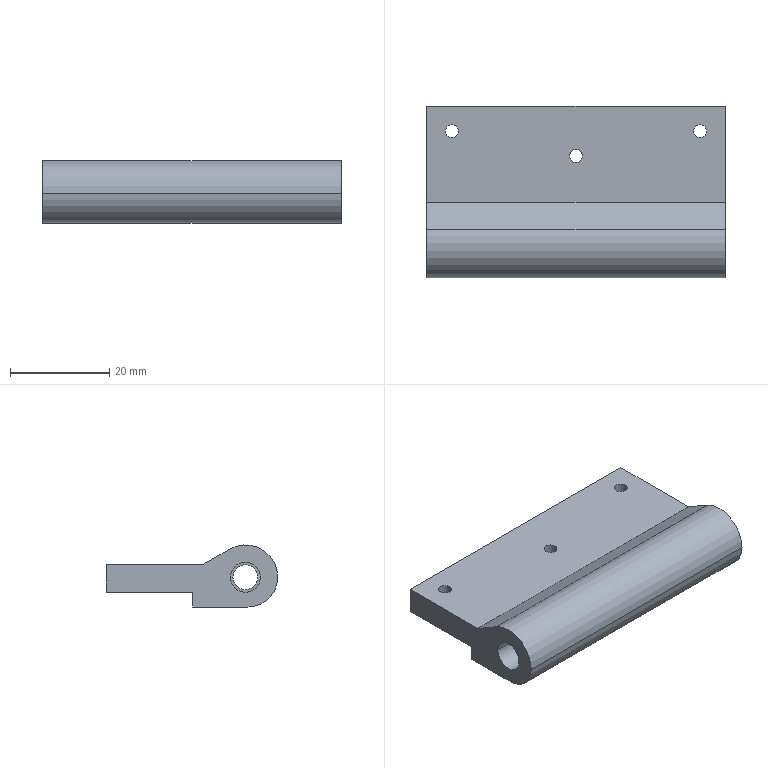Part | NX | 1 solid | 30 faces | box 60 x 34.5 x 12.5 mm | volume 14807 mm3 | cylinder 14 | plane 10 | cone 6 | commonest cylinder face diameters 2.6 x6 6.02 x4 5 x2 12 x1 13 x1
STEP:
#1=CARTESIAN_POINT('',(-23.7,12.25,-4.));
#2=VERTEX_POINT('',#1);
#3=CARTESIAN_POINT('',(-26.3,12.25,-4.));
#4=VERTEX_POINT('',#3);
#5=CARTESIAN_POINT('',(-25.,12.25,-4.));
#6=DIRECTION('',(0.,0.,1.));
#7=DIRECTION('',(1.,0.,0.));
#8=AXIS2_PLACEMENT_3D('',#5,#6,#7);
#9=CIRCLE('',#8,1.3);
#10=EDGE_CURVE('',#2,#4,#9,.T.);
#11=ORIENTED_EDGE('',*,*,#10,.T.);
#12=CARTESIAN_POINT('',(-26.3,12.25,-9.));
#13=VERTEX_POINT('',#12);
#14=CARTESIAN_POINT('',(-26.3,12.25,-10.5));
#15=DIRECTION('',(0.,0.,-1.));
#16=VECTOR('',#15,1000.);
#17=LINE('',#14,#16);
#18=EDGE_CURVE('',#4,#13,#17,.T.);
#19=ORIENTED_EDGE('',*,*,#18,.T.);
#20=CARTESIAN_POINT('',(-23.7,12.25,-9.));
#21=VERTEX_POINT('',#20);
#22=CARTESIAN_POINT('',(-25.,12.25,-9.));
#23=DIRECTION('',(0.,0.,1.));
#24=DIRECTION('',(1.,0.,0.));
#25=AXIS2_PLACEMENT_3D('',#22,#23,#24);
#26=CIRCLE('',#25,1.3);
#27=EDGE_CURVE('',#21,#13,#26,.T.);
#28=ORIENTED_EDGE('',*,*,#27,.F.);
#29=CARTESIAN_POINT('',(-23.7,12.25,-10.5));
#30=DIRECTION('',(0.,0.,-1.));
#31=VECTOR('',#30,1000.);
#32=LINE('',#29,#31);
#33=EDGE_CURVE('',#2,#21,#32,.T.);
#34=ORIENTED_EDGE('',*,*,#33,.F.);
#35=EDGE_LOOP('',(#11,#19,#28,#34));
#36=FACE_BOUND('',#35,.T.);
#37=CARTESIAN_POINT('',(-25.,12.25,-10.5));
#38=DIRECTION('',(0.,0.,-1.));
#39=DIRECTION('',(-1.,0.,0.));
#40=AXIS2_PLACEMENT_3D('',#37,#38,#39);
#41=CYLINDRICAL_SURFACE('',#40,1.3);
#42=ADVANCED_FACE('',(#36),#41,.F.);
#43=CARTESIAN_POINT('',(1.3,7.25,-4.));
#44=VERTEX_POINT('',#43);
#45=CARTESIAN_POINT('',(-1.3,7.25,-4.));
#46=VERTEX_POINT('',#45);
#47=CARTESIAN_POINT('',(0.,7.25,-4.));
#48=DIRECTION('',(0.,0.,1.));
#49=DIRECTION('',(1.,0.,0.));
#50=AXIS2_PLACEMENT_3D('',#47,#48,#49);
#51=CIRCLE('',#50,1.3);
#52=EDGE_CURVE('',#44,#46,#51,.T.);
#53=ORIENTED_EDGE('',*,*,#52,.T.);
#54=CARTESIAN_POINT('',(-1.3,7.25,-9.));
#55=VERTEX_POINT('',#54);
#56=CARTESIAN_POINT('',(-1.3,7.25,-10.5));
#57=DIRECTION('',(0.,0.,-1.));
#58=VECTOR('',#57,1000.);
#59=LINE('',#56,#58);
#60=EDGE_CURVE('',#46,#55,#59,.T.);
#61=ORIENTED_EDGE('',*,*,#60,.T.);
#62=CARTESIAN_POINT('',(1.3,7.25,-9.));
#63=VERTEX_POINT('',#62);
#64=CARTESIAN_POINT('',(0.,7.25,-9.));
#65=DIRECTION('',(0.,0.,1.));
#66=DIRECTION('',(1.,0.,0.));
#67=AXIS2_PLACEMENT_3D('',#64,#65,#66);
#68=CIRCLE('',#67,1.3);
#69=EDGE_CURVE('',#63,#55,#68,.T.);
#70=ORIENTED_EDGE('',*,*,#69,.F.);
#71=CARTESIAN_POINT('',(1.3,7.25,-10.5));
#72=DIRECTION('',(0.,0.,-1.));
#73=VECTOR('',#72,1000.);
#74=LINE('',#71,#73);
#75=EDGE_CURVE('',#44,#63,#74,.T.);
#76=ORIENTED_EDGE('',*,*,#75,.F.);
#77=EDGE_LOOP('',(#53,#61,#70,#76));
#78=FACE_BOUND('',#77,.T.);
#79=CARTESIAN_POINT('',(0.,7.25,-10.5));
#80=DIRECTION('',(0.,0.,-1.));
#81=DIRECTION('',(-1.,0.,0.));
#82=AXIS2_PLACEMENT_3D('',#79,#80,#81);
#83=CYLINDRICAL_SURFACE('',#82,1.3);
#84=ADVANCED_FACE('',(#78),#83,.F.);
#85=CARTESIAN_POINT('',(26.3,12.25,-4.));
#86=VERTEX_POINT('',#85);
#87=CARTESIAN_POINT('',(23.7,12.25,-4.));
#88=VERTEX_POINT('',#87);
#89=CARTESIAN_POINT('',(25.,12.25,-4.));
#90=DIRECTION('',(0.,0.,1.));
#91=DIRECTION('',(1.,0.,0.));
#92=AXIS2_PLACEMENT_3D('',#89,#90,#91);
#93=CIRCLE('',#92,1.3);
#94=EDGE_CURVE('',#86,#88,#93,.T.);
#95=ORIENTED_EDGE('',*,*,#94,.T.);
#96=CARTESIAN_POINT('',(23.7,12.25,-9.));
#97=VERTEX_POINT('',#96);
#98=CARTESIAN_POINT('',(23.7,12.25,-10.5));
#99=DIRECTION('',(0.,0.,-1.));
#100=VECTOR('',#99,1000.);
#101=LINE('',#98,#100);
#102=EDGE_CURVE('',#88,#97,#101,.T.);
#103=ORIENTED_EDGE('',*,*,#102,.T.);
#104=CARTESIAN_POINT('',(26.3,12.25,-9.));
#105=VERTEX_POINT('',#104);
#106=CARTESIAN_POINT('',(25.,12.25,-9.));
#107=DIRECTION('',(0.,0.,1.));
#108=DIRECTION('',(1.,0.,0.));
#109=AXIS2_PLACEMENT_3D('',#106,#107,#108);
#110=CIRCLE('',#109,1.3);
#111=EDGE_CURVE('',#105,#97,#110,.T.);
#112=ORIENTED_EDGE('',*,*,#111,.F.);
#113=CARTESIAN_POINT('',(26.3,12.25,-10.5));
#114=DIRECTION('',(0.,0.,-1.));
#115=VECTOR('',#114,1000.);
#116=LINE('',#113,#115);
#117=EDGE_CURVE('',#86,#105,#116,.T.);
#118=ORIENTED_EDGE('',*,*,#117,.F.);
#119=EDGE_LOOP('',(#95,#103,#112,#118));
#120=FACE_BOUND('',#119,.T.);
#121=CARTESIAN_POINT('',(25.,12.25,-10.5));
#122=DIRECTION('',(0.,0.,-1.));
#123=DIRECTION('',(-1.,0.,0.));
#124=AXIS2_PLACEMENT_3D('',#121,#122,#123);
#125=CYLINDRICAL_SURFACE('',#124,1.3);
#126=ADVANCED_FACE('',(#120),#125,.F.);
#127=ORIENTED_EDGE('',*,*,#27,.T.);
#128=CARTESIAN_POINT('',(-26.8,12.25,-9.5));
#129=VERTEX_POINT('',#128);
#130=CARTESIAN_POINT('',(-26.8,12.25,-9.5));
#131=DIRECTION('',(-0.7071,0.,-0.7071));
#132=VECTOR('',#131,1000.);
#133=LINE('',#130,#132);
#134=EDGE_CURVE('',#13,#129,#133,.T.);
#135=ORIENTED_EDGE('',*,*,#134,.T.);
#136=CARTESIAN_POINT('',(-23.2,12.25,-9.5));
#137=VERTEX_POINT('',#136);
#138=CARTESIAN_POINT('',(-25.,12.25,-9.5));
#139=DIRECTION('',(0.,0.,1.));
#140=DIRECTION('',(1.,0.,0.));
#141=AXIS2_PLACEMENT_3D('',#138,#139,#140);
#142=CIRCLE('',#141,1.8);
#143=EDGE_CURVE('',#137,#129,#142,.T.);
#144=ORIENTED_EDGE('',*,*,#143,.F.);
#145=CARTESIAN_POINT('',(-23.2,12.25,-9.5));
#146=DIRECTION('',(0.7071,0.,-0.7071));
#147=VECTOR('',#146,1000.);
#148=LINE('',#145,#147);
#149=EDGE_CURVE('',#21,#137,#148,.T.);
#150=ORIENTED_EDGE('',*,*,#149,.F.);
#151=EDGE_LOOP('',(#127,#135,#144,#150));
#152=FACE_BOUND('',#151,.T.);
#153=CARTESIAN_POINT('',(-25.,12.25,-9.5));
#154=DIRECTION('',(0.,0.,-1.));
#155=DIRECTION('',(-1.,0.,0.));
#156=AXIS2_PLACEMENT_3D('',#153,#154,#155);
#157=CONICAL_SURFACE('',#156,1.8,0.7854);
#158=ADVANCED_FACE('',(#152),#157,.F.);
#159=ORIENTED_EDGE('',*,*,#69,.T.);
#160=CARTESIAN_POINT('',(-1.8,7.25,-9.5));
#161=VERTEX_POINT('',#160);
#162=CARTESIAN_POINT('',(-1.8,7.25,-9.5));
#163=DIRECTION('',(-0.7071,0.,-0.7071));
#164=VECTOR('',#163,1000.);
#165=LINE('',#162,#164);
#166=EDGE_CURVE('',#55,#161,#165,.T.);
#167=ORIENTED_EDGE('',*,*,#166,.T.);
#168=CARTESIAN_POINT('',(1.8,7.25,-9.5));
#169=VERTEX_POINT('',#168);
#170=CARTESIAN_POINT('',(0.,7.25,-9.5));
#171=DIRECTION('',(0.,0.,1.));
#172=DIRECTION('',(1.,0.,0.));
#173=AXIS2_PLACEMENT_3D('',#170,#171,#172);
#174=CIRCLE('',#173,1.8);
#175=EDGE_CURVE('',#169,#161,#174,.T.);
#176=ORIENTED_EDGE('',*,*,#175,.F.);
#177=CARTESIAN_POINT('',(1.8,7.25,-9.5));
#178=DIRECTION('',(0.7071,0.,-0.7071));
#179=VECTOR('',#178,1000.);
#180=LINE('',#177,#179);
#181=EDGE_CURVE('',#63,#169,#180,.T.);
#182=ORIENTED_EDGE('',*,*,#181,.F.);
#183=EDGE_LOOP('',(#159,#167,#176,#182));
#184=FACE_BOUND('',#183,.T.);
#185=CARTESIAN_POINT('',(0.,7.25,-9.5));
#186=DIRECTION('',(0.,0.,-1.));
#187=DIRECTION('',(-1.,0.,0.));
#188=AXIS2_PLACEMENT_3D('',#185,#186,#187);
#189=CONICAL_SURFACE('',#188,1.8,0.7854);
#190=ADVANCED_FACE('',(#184),#189,.F.);
#191=ORIENTED_EDGE('',*,*,#111,.T.);
#192=CARTESIAN_POINT('',(23.2,12.25,-9.5));
#193=VERTEX_POINT('',#192);
#194=CARTESIAN_POINT('',(23.2,12.25,-9.5));
#195=DIRECTION('',(-0.7071,0.,-0.7071));
#196=VECTOR('',#195,1000.);
#197=LINE('',#194,#196);
#198=EDGE_CURVE('',#97,#193,#197,.T.);
#199=ORIENTED_EDGE('',*,*,#198,.T.);
#200=CARTESIAN_POINT('',(26.8,12.25,-9.5));
#201=VERTEX_POINT('',#200);
#202=CARTESIAN_POINT('',(25.,12.25,-9.5));
#203=DIRECTION('',(0.,0.,1.));
#204=DIRECTION('',(1.,0.,0.));
#205=AXIS2_PLACEMENT_3D('',#202,#203,#204);
#206=CIRCLE('',#205,1.8);
#207=EDGE_CURVE('',#201,#193,#206,.T.);
#208=ORIENTED_EDGE('',*,*,#207,.F.);
#209=CARTESIAN_POINT('',(26.8,12.25,-9.5));
#210=DIRECTION('',(0.7071,0.,-0.7071));
#211=VECTOR('',#210,1000.);
#212=LINE('',#209,#211);
#213=EDGE_CURVE('',#105,#201,#212,.T.);
#214=ORIENTED_EDGE('',*,*,#213,.F.);
#215=EDGE_LOOP('',(#191,#199,#208,#214));
#216=FACE_BOUND('',#215,.T.);
#217=CARTESIAN_POINT('',(25.,12.25,-9.5));
#218=DIRECTION('',(0.,0.,-1.));
#219=DIRECTION('',(-1.,0.,0.));
#220=AXIS2_PLACEMENT_3D('',#217,#218,#219);
#221=CONICAL_SURFACE('',#220,1.8,0.7854);
#222=ADVANCED_FACE('',(#216),#221,.F.);
#223=CARTESIAN_POINT('',(-30.,-13.76,-6.5));
#224=VERTEX_POINT('',#223);
#225=CARTESIAN_POINT('',(-30.,-7.74,-6.5));
#226=VERTEX_POINT('',#225);
#227=CARTESIAN_POINT('',(-30.,-10.75,-6.5));
#228=DIRECTION('',(-1.,0.,0.));
#229=DIRECTION('',(0.,-1.,0.));
#230=AXIS2_PLACEMENT_3D('',#227,#228,#229);
#231=CIRCLE('',#230,3.01);
#232=EDGE_CURVE('',#224,#226,#231,.T.);
#233=ORIENTED_EDGE('',*,*,#232,.T.);
#234=CARTESIAN_POINT('',(-20.2,-7.74,-6.5));
#235=VERTEX_POINT('',#234);
#236=CARTESIAN_POINT('',(-30.,-7.74,-6.5));
#237=DIRECTION('',(1.,0.,0.));
#238=VECTOR('',#237,1000.);
#239=LINE('',#236,#238);
#240=EDGE_CURVE('',#235,#226,#239,.F.);
#241=ORIENTED_EDGE('',*,*,#240,.F.);
#242=CARTESIAN_POINT('',(-20.2,-13.76,-6.5));
#243=VERTEX_POINT('',#242);
#244=CARTESIAN_POINT('',(-20.2,-10.75,-6.5));
#245=DIRECTION('',(-1.,0.,0.));
#246=DIRECTION('',(0.,-1.,0.));
#247=AXIS2_PLACEMENT_3D('',#244,#245,#246);
#248=CIRCLE('',#247,3.01);
#249=EDGE_CURVE('',#243,#235,#248,.T.);
#250=ORIENTED_EDGE('',*,*,#249,.F.);
#251=CARTESIAN_POINT('',(-30.,-13.76,-6.5));
#252=DIRECTION('',(1.,0.,0.));
#253=VECTOR('',#252,1000.);
#254=LINE('',#251,#253);
#255=EDGE_CURVE('',#243,#224,#254,.F.);
#256=ORIENTED_EDGE('',*,*,#255,.T.);
#257=EDGE_LOOP('',(#233,#241,#250,#256));
#258=FACE_BOUND('',#257,.T.);
#259=CARTESIAN_POINT('',(-30.,-10.75,-6.5));
#260=DIRECTION('',(1.,0.,0.));
#261=DIRECTION('',(0.,1.,0.));
#262=AXIS2_PLACEMENT_3D('',#259,#260,#261);
#263=CYLINDRICAL_SURFACE('',#262,3.01);
#264=ADVANCED_FACE('',(#258),#263,.F.);
#265=CARTESIAN_POINT('',(20.2,-7.74,-6.5));
#266=VERTEX_POINT('',#265);
#267=CARTESIAN_POINT('',(20.2,-13.76,-6.5));
#268=VERTEX_POINT('',#267);
#269=CARTESIAN_POINT('',(20.2,-10.75,-6.5));
#270=DIRECTION('',(1.,0.,0.));
#271=DIRECTION('',(0.,-1.,0.));
#272=AXIS2_PLACEMENT_3D('',#269,#270,#271);
#273=CIRCLE('',#272,3.01);
#274=EDGE_CURVE('',#266,#268,#273,.T.);
#275=ORIENTED_EDGE('',*,*,#274,.F.);
#276=CARTESIAN_POINT('',(30.,-7.74,-6.5));
#277=VERTEX_POINT('',#276);
#278=CARTESIAN_POINT('',(30.,-7.74,-6.5));
#279=DIRECTION('',(1.,0.,0.));
#280=VECTOR('',#279,1000.);
#281=LINE('',#278,#280);
#282=EDGE_CURVE('',#277,#266,#281,.F.);
#283=ORIENTED_EDGE('',*,*,#282,.F.);
#284=CARTESIAN_POINT('',(30.,-13.76,-6.5));
#285=VERTEX_POINT('',#284);
#286=CARTESIAN_POINT('',(30.,-10.75,-6.5));
#287=DIRECTION('',(1.,0.,0.));
#288=DIRECTION('',(0.,-1.,0.));
#289=AXIS2_PLACEMENT_3D('',#286,#287,#288);
#290=CIRCLE('',#289,3.01);
#291=EDGE_CURVE('',#277,#285,#290,.T.);
#292=ORIENTED_EDGE('',*,*,#291,.T.);
#293=CARTESIAN_POINT('',(30.,-13.76,-6.5));
#294=DIRECTION('',(1.,0.,0.));
#295=VECTOR('',#294,1000.);
#296=LINE('',#293,#295);
#297=EDGE_CURVE('',#285,#268,#296,.F.);
#298=ORIENTED_EDGE('',*,*,#297,.T.);
#299=EDGE_LOOP('',(#275,#283,#292,#298));
#300=FACE_BOUND('',#299,.T.);
#301=CARTESIAN_POINT('',(30.,-10.75,-6.5));
#302=DIRECTION('',(1.,0.,0.));
#303=DIRECTION('',(0.,1.,0.));
#304=AXIS2_PLACEMENT_3D('',#301,#302,#303);
#305=CYLINDRICAL_SURFACE('',#304,3.01);
#306=ADVANCED_FACE('',(#300),#305,.F.);
#307=CARTESIAN_POINT('',(-20.2,-13.25,-6.5));
#308=VERTEX_POINT('',#307);
#309=CARTESIAN_POINT('',(-20.2,-8.25,-6.5));
#310=VERTEX_POINT('',#309);
#311=CARTESIAN_POINT('',(-20.2,-10.75,-6.5));
#312=DIRECTION('',(-1.,0.,0.));
#313=DIRECTION('',(0.,-1.,0.));
#314=AXIS2_PLACEMENT_3D('',#311,#312,#313);
#315=CIRCLE('',#314,2.5);
#316=EDGE_CURVE('',#308,#310,#315,.T.);
#317=ORIENTED_EDGE('',*,*,#316,.T.);
#318=CARTESIAN_POINT('',(20.2,-8.25,-6.5));
#319=VERTEX_POINT('',#318);
#320=CARTESIAN_POINT('',(30.,-8.25,-6.5));
#321=DIRECTION('',(1.,0.,0.));
#322=VECTOR('',#321,1000.);
#323=LINE('',#320,#322);
#324=EDGE_CURVE('',#319,#310,#323,.F.);
#325=ORIENTED_EDGE('',*,*,#324,.F.);
#326=CARTESIAN_POINT('',(20.2,-13.25,-6.5));
#327=VERTEX_POINT('',#326);
#328=CARTESIAN_POINT('',(20.2,-10.75,-6.5));
#329=DIRECTION('',(-1.,0.,0.));
#330=DIRECTION('',(0.,-1.,0.));
#331=AXIS2_PLACEMENT_3D('',#328,#329,#330);
#332=CIRCLE('',#331,2.5);
#333=EDGE_CURVE('',#327,#319,#332,.T.);
#334=ORIENTED_EDGE('',*,*,#333,.F.);
#335=CARTESIAN_POINT('',(30.,-13.25,-6.5));
#336=DIRECTION('',(1.,0.,0.));
#337=VECTOR('',#336,1000.);
#338=LINE('',#335,#337);
#339=EDGE_CURVE('',#327,#308,#338,.F.);
#340=ORIENTED_EDGE('',*,*,#339,.T.);
#341=EDGE_LOOP('',(#317,#325,#334,#340));
#342=FACE_BOUND('',#341,.T.);
#343=CARTESIAN_POINT('',(30.,-10.75,-6.5));
#344=DIRECTION('',(1.,0.,0.));
#345=DIRECTION('',(0.,1.,0.));
#346=AXIS2_PLACEMENT_3D('',#343,#344,#345);
#347=CYLINDRICAL_SURFACE('',#346,2.5);
#348=ADVANCED_FACE('',(#342),#347,.F.);
#349=ORIENTED_EDGE('',*,*,#10,.F.);
#350=CARTESIAN_POINT('',(-25.,12.25,-4.));
#351=DIRECTION('',(0.,0.,1.));
#352=DIRECTION('',(1.,0.,0.));
#353=AXIS2_PLACEMENT_3D('',#350,#351,#352);
#354=CIRCLE('',#353,1.3);
#355=EDGE_CURVE('',#4,#2,#354,.T.);
#356=ORIENTED_EDGE('',*,*,#355,.F.);
#357=EDGE_LOOP('',(#349,#356));
#358=FACE_BOUND('',#357,.T.);
#359=ORIENTED_EDGE('',*,*,#52,.F.);
#360=CARTESIAN_POINT('',(0.,7.25,-4.));
#361=DIRECTION('',(0.,0.,1.));
#362=DIRECTION('',(1.,0.,0.));
#363=AXIS2_PLACEMENT_3D('',#360,#361,#362);
#364=CIRCLE('',#363,1.3);
#365=EDGE_CURVE('',#46,#44,#364,.T.);
#366=ORIENTED_EDGE('',*,*,#365,.F.);
#367=EDGE_LOOP('',(#359,#366));
#368=FACE_BOUND('',#367,.T.);
#369=ORIENTED_EDGE('',*,*,#94,.F.);
#370=CARTESIAN_POINT('',(25.,12.25,-4.));
#371=DIRECTION('',(0.,0.,1.));
#372=DIRECTION('',(1.,0.,0.));
#373=AXIS2_PLACEMENT_3D('',#370,#371,#372);
#374=CIRCLE('',#373,1.3);
#375=EDGE_CURVE('',#88,#86,#374,.T.);
#376=ORIENTED_EDGE('',*,*,#375,.F.);
#377=EDGE_LOOP('',(#369,#376));
#378=FACE_BOUND('',#377,.T.);
#379=CARTESIAN_POINT('',(30.,-2.08,-4.));
#380=VERTEX_POINT('',#379);
#381=CARTESIAN_POINT('',(-30.,-2.08,-4.));
#382=VERTEX_POINT('',#381);
#383=CARTESIAN_POINT('',(30.,-2.08,-4.));
#384=DIRECTION('',(-1.,0.,0.));
#385=VECTOR('',#384,1000.);
#386=LINE('',#383,#385);
#387=EDGE_CURVE('',#380,#382,#386,.T.);
#388=ORIENTED_EDGE('',*,*,#387,.F.);
#389=CARTESIAN_POINT('',(30.,17.25,-4.));
#390=VERTEX_POINT('',#389);
#391=CARTESIAN_POINT('',(30.,-2.08,-4.));
#392=DIRECTION('',(0.,-1.,0.));
#393=VECTOR('',#392,1000.);
#394=LINE('',#391,#393);
#395=EDGE_CURVE('',#390,#380,#394,.T.);
#396=ORIENTED_EDGE('',*,*,#395,.F.);
#397=CARTESIAN_POINT('',(-30.,17.25,-4.));
#398=VERTEX_POINT('',#397);
#399=CARTESIAN_POINT('',(30.,17.25,-4.));
#400=DIRECTION('',(1.,0.,0.));
#401=VECTOR('',#400,1000.);
#402=LINE('',#399,#401);
#403=EDGE_CURVE('',#398,#390,#402,.T.);
#404=ORIENTED_EDGE('',*,*,#403,.F.);
#405=CARTESIAN_POINT('',(-30.,-2.08,-4.));
#406=DIRECTION('',(0.,1.,0.));
#407=VECTOR('',#406,1000.);
#408=LINE('',#405,#407);
#409=EDGE_CURVE('',#382,#398,#408,.T.);
#410=ORIENTED_EDGE('',*,*,#409,.F.);
#411=EDGE_LOOP('',(#388,#396,#404,#410));
#412=FACE_BOUND('',#411,.T.);
#413=CARTESIAN_POINT('',(30.,-2.08,-4.));
#414=DIRECTION('',(0.,0.,-1.));
#415=DIRECTION('',(-1.,0.,0.));
#416=AXIS2_PLACEMENT_3D('',#413,#414,#415);
#417=PLANE('',#416);
#418=ADVANCED_FACE('',(#358,#368,#378,#412),#417,.F.);
#419=ORIENTED_EDGE('',*,*,#18,.F.);
#420=ORIENTED_EDGE('',*,*,#355,.T.);
#421=ORIENTED_EDGE('',*,*,#33,.T.);
#422=CARTESIAN_POINT('',(-25.,12.25,-9.));
#423=DIRECTION('',(0.,0.,1.));
#424=DIRECTION('',(1.,0.,0.));
#425=AXIS2_PLACEMENT_3D('',#422,#423,#424);
#426=CIRCLE('',#425,1.3);
#427=EDGE_CURVE('',#13,#21,#426,.T.);
#428=ORIENTED_EDGE('',*,*,#427,.F.);
#429=EDGE_LOOP('',(#419,#420,#421,#428));
#430=FACE_BOUND('',#429,.T.);
#431=CARTESIAN_POINT('',(-25.,12.25,-10.5));
#432=DIRECTION('',(0.,0.,-1.));
#433=DIRECTION('',(-1.,0.,0.));
#434=AXIS2_PLACEMENT_3D('',#431,#432,#433);
#435=CYLINDRICAL_SURFACE('',#434,1.3);
#436=ADVANCED_FACE('',(#430),#435,.F.);
#437=ORIENTED_EDGE('',*,*,#60,.F.);
#438=ORIENTED_EDGE('',*,*,#365,.T.);
#439=ORIENTED_EDGE('',*,*,#75,.T.);
#440=CARTESIAN_POINT('',(0.,7.25,-9.));
#441=DIRECTION('',(0.,0.,1.));
#442=DIRECTION('',(1.,0.,0.));
#443=AXIS2_PLACEMENT_3D('',#440,#441,#442);
#444=CIRCLE('',#443,1.3);
#445=EDGE_CURVE('',#55,#63,#444,.T.);
#446=ORIENTED_EDGE('',*,*,#445,.F.);
#447=EDGE_LOOP('',(#437,#438,#439,#446));
#448=FACE_BOUND('',#447,.T.);
#449=CARTESIAN_POINT('',(0.,7.25,-10.5));
#450=DIRECTION('',(0.,0.,-1.));
#451=DIRECTION('',(-1.,0.,0.));
#452=AXIS2_PLACEMENT_3D('',#449,#450,#451);
#453=CYLINDRICAL_SURFACE('',#452,1.3);
#454=ADVANCED_FACE('',(#448),#453,.F.);
#455=ORIENTED_EDGE('',*,*,#102,.F.);
#456=ORIENTED_EDGE('',*,*,#375,.T.);
#457=ORIENTED_EDGE('',*,*,#117,.T.);
#458=CARTESIAN_POINT('',(25.,12.25,-9.));
#459=DIRECTION('',(0.,0.,1.));
#460=DIRECTION('',(1.,0.,0.));
#461=AXIS2_PLACEMENT_3D('',#458,#459,#460);
#462=CIRCLE('',#461,1.3);
#463=EDGE_CURVE('',#97,#105,#462,.T.);
#464=ORIENTED_EDGE('',*,*,#463,.F.);
#465=EDGE_LOOP('',(#455,#456,#457,#464));
#466=FACE_BOUND('',#465,.T.);
#467=CARTESIAN_POINT('',(25.,12.25,-10.5));
#468=DIRECTION('',(0.,0.,-1.));
#469=DIRECTION('',(-1.,0.,0.));
#470=AXIS2_PLACEMENT_3D('',#467,#468,#469);
#471=CYLINDRICAL_SURFACE('',#470,1.3);
#472=ADVANCED_FACE('',(#466),#471,.F.);
#473=ORIENTED_EDGE('',*,*,#232,.F.);
#474=CARTESIAN_POINT('',(-30.,-10.75,-6.5));
#475=DIRECTION('',(-1.,0.,0.));
#476=DIRECTION('',(0.,-1.,0.));
#477=AXIS2_PLACEMENT_3D('',#474,#475,#476);
#478=CIRCLE('',#477,3.01);
#479=EDGE_CURVE('',#226,#224,#478,.T.);
#480=ORIENTED_EDGE('',*,*,#479,.F.);
#481=EDGE_LOOP('',(#473,#480));
#482=FACE_BOUND('',#481,.T.);
#483=CARTESIAN_POINT('',(-30.,-0.15,-12.5));
#484=VERTEX_POINT('',#483);
#485=CARTESIAN_POINT('',(-30.,-0.15,-9.5));
#486=VERTEX_POINT('',#485);
#487=CARTESIAN_POINT('',(-30.,-0.15,-10.5));
#488=DIRECTION('',(0.,0.,1.));
#489=VECTOR('',#488,1000.);
#490=LINE('',#487,#489);
#491=EDGE_CURVE('',#484,#486,#490,.T.);
#492=ORIENTED_EDGE('',*,*,#491,.F.);
#493=CARTESIAN_POINT('',(-30.,-11.25,-12.5));
#494=VERTEX_POINT('',#493);
#495=CARTESIAN_POINT('',(-30.,214.25,-12.5));
#496=DIRECTION('',(0.,1.,0.));
#497=VECTOR('',#496,1000.);
#498=LINE('',#495,#497);
#499=EDGE_CURVE('',#494,#484,#498,.T.);
#500=ORIENTED_EDGE('',*,*,#499,.F.);
#501=CARTESIAN_POINT('',(-30.,-17.25,-6.5));
#502=VERTEX_POINT('',#501);
#503=CARTESIAN_POINT('',(-30.,-11.25,-6.5));
#504=DIRECTION('',(1.,0.,0.));
#505=DIRECTION('',(0.,1.,0.));
#506=AXIS2_PLACEMENT_3D('',#503,#504,#505);
#507=CIRCLE('',#506,6.);
#508=EDGE_CURVE('',#502,#494,#507,.T.);
#509=ORIENTED_EDGE('',*,*,#508,.F.);
#510=CARTESIAN_POINT('',(-30.,-7.5,-0.8708));
#511=VERTEX_POINT('',#510);
#512=CARTESIAN_POINT('',(-30.,-10.75,-6.5));
#513=DIRECTION('',(1.,0.,0.));
#514=DIRECTION('',(0.,-1.,0.));
#515=AXIS2_PLACEMENT_3D('',#512,#513,#514);
#516=CIRCLE('',#515,6.5);
#517=EDGE_CURVE('',#511,#502,#516,.T.);
#518=ORIENTED_EDGE('',*,*,#517,.F.);
#519=CARTESIAN_POINT('',(-30.,-2.08,-4.));
#520=DIRECTION('',(0.,-0.866,0.5));
#521=VECTOR('',#520,1000.);
#522=LINE('',#519,#521);
#523=EDGE_CURVE('',#382,#511,#522,.T.);
#524=ORIENTED_EDGE('',*,*,#523,.F.);
#525=ORIENTED_EDGE('',*,*,#409,.T.);
#526=CARTESIAN_POINT('',(-30.,17.25,-9.5));
#527=VERTEX_POINT('',#526);
#528=CARTESIAN_POINT('',(-30.,17.25,120.5));
#529=DIRECTION('',(0.,0.,1.));
#530=VECTOR('',#529,1000.);
#531=LINE('',#528,#530);
#532=EDGE_CURVE('',#527,#398,#531,.T.);
#533=ORIENTED_EDGE('',*,*,#532,.F.);
#534=CARTESIAN_POINT('',(-30.,214.25,-9.5));
#535=DIRECTION('',(0.,1.,0.));
#536=VECTOR('',#535,1000.);
#537=LINE('',#534,#536);
#538=EDGE_CURVE('',#486,#527,#537,.T.);
#539=ORIENTED_EDGE('',*,*,#538,.F.);
#540=EDGE_LOOP('',(#492,#500,#509,#518,#524,#525,#533,#539));
#541=FACE_BOUND('',#540,.T.);
#542=CARTESIAN_POINT('',(-30.,214.25,120.5));
#543=DIRECTION('',(1.,0.,0.));
#544=DIRECTION('',(0.,1.,0.));
#545=AXIS2_PLACEMENT_3D('',#542,#543,#544);
#546=PLANE('',#545);
#547=ADVANCED_FACE('',(#482,#541),#546,.F.);
#548=ORIENTED_EDGE('',*,*,#387,.T.);
#549=ORIENTED_EDGE('',*,*,#523,.T.);
#550=CARTESIAN_POINT('',(30.,-7.5,-0.8708));
#551=VERTEX_POINT('',#550);
#552=CARTESIAN_POINT('',(30.,-7.5,-0.8708));
#553=DIRECTION('',(-1.,0.,0.));
#554=VECTOR('',#553,1000.);
#555=LINE('',#552,#554);
#556=EDGE_CURVE('',#551,#511,#555,.T.);
#557=ORIENTED_EDGE('',*,*,#556,.F.);
#558=CARTESIAN_POINT('',(30.,-7.5,-0.8708));
#559=DIRECTION('',(0.,-0.866,0.5));
#560=VECTOR('',#559,1000.);
#561=LINE('',#558,#560);
#562=EDGE_CURVE('',#380,#551,#561,.T.);
#563=ORIENTED_EDGE('',*,*,#562,.F.);
#564=EDGE_LOOP('',(#548,#549,#557,#563));
#565=FACE_BOUND('',#564,.T.);
#566=CARTESIAN_POINT('',(30.,-7.5,-0.8708));
#567=DIRECTION('',(0.,-0.5,-0.866));
#568=DIRECTION('',(0.,-0.866,0.5));
#569=AXIS2_PLACEMENT_3D('',#566,#567,#568);
#570=PLANE('',#569);
#571=ADVANCED_FACE('',(#565),#570,.F.);
#572=CARTESIAN_POINT('',(30.,-10.75,-6.5));
#573=DIRECTION('',(1.,0.,0.));
#574=DIRECTION('',(0.,-1.,0.));
#575=AXIS2_PLACEMENT_3D('',#572,#573,#574);
#576=CIRCLE('',#575,3.01);
#577=EDGE_CURVE('',#285,#277,#576,.T.);
#578=ORIENTED_EDGE('',*,*,#577,.F.);
#579=ORIENTED_EDGE('',*,*,#291,.F.);
#580=EDGE_LOOP('',(#578,#579));
#581=FACE_BOUND('',#580,.T.);
#582=ORIENTED_EDGE('',*,*,#562,.T.);
#583=CARTESIAN_POINT('',(30.,-17.25,-6.5));
#584=VERTEX_POINT('',#583);
#585=CARTESIAN_POINT('',(30.,-10.75,-6.5));
#586=DIRECTION('',(-1.,0.,0.));
#587=DIRECTION('',(0.,-1.,0.));
#588=AXIS2_PLACEMENT_3D('',#585,#586,#587);
#589=CIRCLE('',#588,6.5);
#590=EDGE_CURVE('',#584,#551,#589,.T.);
#591=ORIENTED_EDGE('',*,*,#590,.F.);
#592=CARTESIAN_POINT('',(30.,-11.25,-12.5));
#593=VERTEX_POINT('',#592);
#594=CARTESIAN_POINT('',(30.,-11.25,-6.5));
#595=DIRECTION('',(-1.,0.,0.));
#596=DIRECTION('',(0.,1.,0.));
#597=AXIS2_PLACEMENT_3D('',#594,#595,#596);
#598=CIRCLE('',#597,6.);
#599=EDGE_CURVE('',#593,#584,#598,.T.);
#600=ORIENTED_EDGE('',*,*,#599,.F.);
#601=CARTESIAN_POINT('',(30.,-0.15,-12.5));
#602=VERTEX_POINT('',#601);
#603=CARTESIAN_POINT('',(30.,214.25,-12.5));
#604=DIRECTION('',(0.,-1.,0.));
#605=VECTOR('',#604,1000.);
#606=LINE('',#603,#605);
#607=EDGE_CURVE('',#602,#593,#606,.T.);
#608=ORIENTED_EDGE('',*,*,#607,.F.);
#609=CARTESIAN_POINT('',(30.,-0.15,-9.5));
#610=VERTEX_POINT('',#609);
#611=CARTESIAN_POINT('',(30.,-0.15,-10.5));
#612=DIRECTION('',(0.,0.,-1.));
#613=VECTOR('',#612,1000.);
#614=LINE('',#611,#613);
#615=EDGE_CURVE('',#610,#602,#614,.T.);
#616=ORIENTED_EDGE('',*,*,#615,.F.);
#617=CARTESIAN_POINT('',(30.,17.25,-9.5));
#618=VERTEX_POINT('',#617);
#619=CARTESIAN_POINT('',(30.,214.25,-9.5));
#620=DIRECTION('',(0.,-1.,0.));
#621=VECTOR('',#620,1000.);
#622=LINE('',#619,#621);
#623=EDGE_CURVE('',#618,#610,#622,.T.);
#624=ORIENTED_EDGE('',*,*,#623,.F.);
#625=CARTESIAN_POINT('',(30.,17.25,-12.5));
#626=DIRECTION('',(0.,0.,-1.));
#627=VECTOR('',#626,1000.);
#628=LINE('',#625,#627);
#629=EDGE_CURVE('',#390,#618,#628,.T.);
#630=ORIENTED_EDGE('',*,*,#629,.F.);
#631=ORIENTED_EDGE('',*,*,#395,.T.);
#632=EDGE_LOOP('',(#582,#591,#600,#608,#616,#624,#630,#631));
#633=FACE_BOUND('',#632,.T.);
#634=CARTESIAN_POINT('',(30.,214.25,-12.5));
#635=DIRECTION('',(-1.,0.,0.));
#636=DIRECTION('',(0.,-1.,0.));
#637=AXIS2_PLACEMENT_3D('',#634,#635,#636);
#638=PLANE('',#637);
#639=ADVANCED_FACE('',(#581,#633),#638,.F.);
#640=ORIENTED_EDGE('',*,*,#532,.T.);
#641=ORIENTED_EDGE('',*,*,#403,.T.);
#642=ORIENTED_EDGE('',*,*,#629,.T.);
#643=CARTESIAN_POINT('',(30.,17.25,-9.5));
#644=DIRECTION('',(-1.,0.,0.));
#645=VECTOR('',#644,1000.);
#646=LINE('',#643,#645);
#647=EDGE_CURVE('',#618,#527,#646,.T.);
#648=ORIENTED_EDGE('',*,*,#647,.T.);
#649=EDGE_LOOP('',(#640,#641,#642,#648));
#650=FACE_BOUND('',#649,.T.);
#651=CARTESIAN_POINT('',(30.,17.25,-10.5));
#652=DIRECTION('',(0.,1.,0.));
#653=DIRECTION('',(-1.,0.,0.));
#654=AXIS2_PLACEMENT_3D('',#651,#652,#653);
#655=PLANE('',#654);
#656=ADVANCED_FACE('',(#650),#655,.T.);
#657=ORIENTED_EDGE('',*,*,#134,.F.);
#658=ORIENTED_EDGE('',*,*,#427,.T.);
#659=ORIENTED_EDGE('',*,*,#149,.T.);
#660=CARTESIAN_POINT('',(-25.,12.25,-9.5));
#661=DIRECTION('',(0.,0.,1.));
#662=DIRECTION('',(1.,0.,0.));
#663=AXIS2_PLACEMENT_3D('',#660,#661,#662);
#664=CIRCLE('',#663,1.8);
#665=EDGE_CURVE('',#129,#137,#664,.T.);
#666=ORIENTED_EDGE('',*,*,#665,.F.);
#667=EDGE_LOOP('',(#657,#658,#659,#666));
#668=FACE_BOUND('',#667,.T.);
#669=CARTESIAN_POINT('',(-25.,12.25,-9.5));
#670=DIRECTION('',(0.,0.,-1.));
#671=DIRECTION('',(-1.,0.,0.));
#672=AXIS2_PLACEMENT_3D('',#669,#670,#671);
#673=CONICAL_SURFACE('',#672,1.8,0.7854);
#674=ADVANCED_FACE('',(#668),#673,.F.);
#675=ORIENTED_EDGE('',*,*,#166,.F.);
#676=ORIENTED_EDGE('',*,*,#445,.T.);
#677=ORIENTED_EDGE('',*,*,#181,.T.);
#678=CARTESIAN_POINT('',(0.,7.25,-9.5));
#679=DIRECTION('',(0.,0.,1.));
#680=DIRECTION('',(1.,0.,0.));
#681=AXIS2_PLACEMENT_3D('',#678,#679,#680);
#682=CIRCLE('',#681,1.8);
#683=EDGE_CURVE('',#161,#169,#682,.T.);
#684=ORIENTED_EDGE('',*,*,#683,.F.);
#685=EDGE_LOOP('',(#675,#676,#677,#684));
#686=FACE_BOUND('',#685,.T.);
#687=CARTESIAN_POINT('',(0.,7.25,-9.5));
#688=DIRECTION('',(0.,0.,-1.));
#689=DIRECTION('',(-1.,0.,0.));
#690=AXIS2_PLACEMENT_3D('',#687,#688,#689);
#691=CONICAL_SURFACE('',#690,1.8,0.7854);
#692=ADVANCED_FACE('',(#686),#691,.F.);
#693=ORIENTED_EDGE('',*,*,#198,.F.);
#694=ORIENTED_EDGE('',*,*,#463,.T.);
#695=ORIENTED_EDGE('',*,*,#213,.T.);
#696=CARTESIAN_POINT('',(25.,12.25,-9.5));
#697=DIRECTION('',(0.,0.,1.));
#698=DIRECTION('',(1.,0.,0.));
#699=AXIS2_PLACEMENT_3D('',#696,#697,#698);
#700=CIRCLE('',#699,1.8);
#701=EDGE_CURVE('',#193,#201,#700,.T.);
#702=ORIENTED_EDGE('',*,*,#701,.F.);
#703=EDGE_LOOP('',(#693,#694,#695,#702));
#704=FACE_BOUND('',#703,.T.);
#705=CARTESIAN_POINT('',(25.,12.25,-9.5));
#706=DIRECTION('',(0.,0.,-1.));
#707=DIRECTION('',(-1.,0.,0.));
#708=AXIS2_PLACEMENT_3D('',#705,#706,#707);
#709=CONICAL_SURFACE('',#708,1.8,0.7854);
#710=ADVANCED_FACE('',(#704),#709,.F.);
#711=ORIENTED_EDGE('',*,*,#240,.T.);
#712=ORIENTED_EDGE('',*,*,#479,.T.);
#713=ORIENTED_EDGE('',*,*,#255,.F.);
#714=CARTESIAN_POINT('',(-20.2,-10.75,-6.5));
#715=DIRECTION('',(-1.,0.,0.));
#716=DIRECTION('',(0.,-1.,0.));
#717=AXIS2_PLACEMENT_3D('',#714,#715,#716);
#718=CIRCLE('',#717,3.01);
#719=EDGE_CURVE('',#235,#243,#718,.T.);
#720=ORIENTED_EDGE('',*,*,#719,.F.);
#721=EDGE_LOOP('',(#711,#712,#713,#720));
#722=FACE_BOUND('',#721,.T.);
#723=CARTESIAN_POINT('',(-30.,-10.75,-6.5));
#724=DIRECTION('',(1.,0.,0.));
#725=DIRECTION('',(0.,1.,0.));
#726=AXIS2_PLACEMENT_3D('',#723,#724,#725);
#727=CYLINDRICAL_SURFACE('',#726,3.01);
#728=ADVANCED_FACE('',(#722),#727,.F.);
#729=ORIENTED_EDGE('',*,*,#207,.T.);
#730=ORIENTED_EDGE('',*,*,#701,.T.);
#731=EDGE_LOOP('',(#729,#730));
#732=FACE_BOUND('',#731,.T.);
#733=ORIENTED_EDGE('',*,*,#175,.T.);
#734=ORIENTED_EDGE('',*,*,#683,.T.);
#735=EDGE_LOOP('',(#733,#734));
#736=FACE_BOUND('',#735,.T.);
#737=ORIENTED_EDGE('',*,*,#143,.T.);
#738=ORIENTED_EDGE('',*,*,#665,.T.);
#739=EDGE_LOOP('',(#737,#738));
#740=FACE_BOUND('',#739,.T.);
#741=CARTESIAN_POINT('',(30.,-0.15,-9.5));
#742=DIRECTION('',(1.,0.,0.));
#743=VECTOR('',#742,1000.);
#744=LINE('',#741,#743);
#745=EDGE_CURVE('',#486,#610,#744,.T.);
#746=ORIENTED_EDGE('',*,*,#745,.F.);
#747=ORIENTED_EDGE('',*,*,#538,.T.);
#748=ORIENTED_EDGE('',*,*,#647,.F.);
#749=ORIENTED_EDGE('',*,*,#623,.T.);
#750=EDGE_LOOP('',(#746,#747,#748,#749));
#751=FACE_BOUND('',#750,.T.);
#752=CARTESIAN_POINT('',(30.,17.25,-9.5));
#753=DIRECTION('',(0.,0.,1.));
#754=DIRECTION('',(1.,0.,0.));
#755=AXIS2_PLACEMENT_3D('',#752,#753,#754);
#756=PLANE('',#755);
#757=ADVANCED_FACE('',(#732,#736,#740,#751),#756,.F.);
#758=ORIENTED_EDGE('',*,*,#745,.T.);
#759=ORIENTED_EDGE('',*,*,#615,.T.);
#760=CARTESIAN_POINT('',(30.,-0.15,-12.5));
#761=DIRECTION('',(1.,0.,0.));
#762=VECTOR('',#761,1000.);
#763=LINE('',#760,#762);
#764=EDGE_CURVE('',#484,#602,#763,.T.);
#765=ORIENTED_EDGE('',*,*,#764,.F.);
#766=ORIENTED_EDGE('',*,*,#491,.T.);
#767=EDGE_LOOP('',(#758,#759,#765,#766));
#768=FACE_BOUND('',#767,.T.);
#769=CARTESIAN_POINT('',(30.,-0.15,-10.5));
#770=DIRECTION('',(0.,-1.,0.));
#771=DIRECTION('',(1.,0.,0.));
#772=AXIS2_PLACEMENT_3D('',#769,#770,#771);
#773=PLANE('',#772);
#774=ADVANCED_FACE('',(#768),#773,.F.);
#775=ORIENTED_EDGE('',*,*,#499,.T.);
#776=ORIENTED_EDGE('',*,*,#764,.T.);
#777=ORIENTED_EDGE('',*,*,#607,.T.);
#778=CARTESIAN_POINT('',(-40.,-11.25,-12.5));
#779=DIRECTION('',(-1.,0.,0.));
#780=VECTOR('',#779,1000.);
#781=LINE('',#778,#780);
#782=EDGE_CURVE('',#593,#494,#781,.T.);
#783=ORIENTED_EDGE('',*,*,#782,.T.);
#784=EDGE_LOOP('',(#775,#776,#777,#783));
#785=FACE_BOUND('',#784,.T.);
#786=CARTESIAN_POINT('',(-40.,-55.75,-12.5));
#787=DIRECTION('',(0.,0.,-1.));
#788=DIRECTION('',(-1.,0.,0.));
#789=AXIS2_PLACEMENT_3D('',#786,#787,#788);
#790=PLANE('',#789);
#791=ADVANCED_FACE('',(#785),#790,.T.);
#792=CARTESIAN_POINT('',(108.216,-17.25,-6.5));
#793=DIRECTION('',(-1.,0.,0.));
#794=VECTOR('',#793,1000.);
#795=LINE('',#792,#794);
#796=EDGE_CURVE('',#584,#502,#795,.T.);
#797=ORIENTED_EDGE('',*,*,#796,.T.);
#798=ORIENTED_EDGE('',*,*,#508,.T.);
#799=ORIENTED_EDGE('',*,*,#782,.F.);
#800=ORIENTED_EDGE('',*,*,#599,.T.);
#801=EDGE_LOOP('',(#797,#798,#799,#800));
#802=FACE_BOUND('',#801,.T.);
#803=CARTESIAN_POINT('',(108.216,-11.25,-6.5));
#804=DIRECTION('',(-1.,0.,0.));
#805=DIRECTION('',(0.,-1.,0.));
#806=AXIS2_PLACEMENT_3D('',#803,#804,#805);
#807=CYLINDRICAL_SURFACE('',#806,6.);
#808=ADVANCED_FACE('',(#802),#807,.T.);
#809=ORIENTED_EDGE('',*,*,#556,.T.);
#810=ORIENTED_EDGE('',*,*,#517,.T.);
#811=ORIENTED_EDGE('',*,*,#796,.F.);
#812=ORIENTED_EDGE('',*,*,#590,.T.);
#813=EDGE_LOOP('',(#809,#810,#811,#812));
#814=FACE_BOUND('',#813,.T.);
#815=CARTESIAN_POINT('',(30.,-10.75,-6.5));
#816=DIRECTION('',(1.,0.,0.));
#817=DIRECTION('',(0.,1.,0.));
#818=AXIS2_PLACEMENT_3D('',#815,#816,#817);
#819=CYLINDRICAL_SURFACE('',#818,6.5);
#820=ADVANCED_FACE('',(#814),#819,.T.);
#821=ORIENTED_EDGE('',*,*,#282,.T.);
#822=CARTESIAN_POINT('',(20.2,-10.75,-6.5));
#823=DIRECTION('',(1.,0.,0.));
#824=DIRECTION('',(0.,-1.,0.));
#825=AXIS2_PLACEMENT_3D('',#822,#823,#824);
#826=CIRCLE('',#825,3.01);
#827=EDGE_CURVE('',#268,#266,#826,.T.);
#828=ORIENTED_EDGE('',*,*,#827,.F.);
#829=ORIENTED_EDGE('',*,*,#297,.F.);
#830=ORIENTED_EDGE('',*,*,#577,.T.);
#831=EDGE_LOOP('',(#821,#828,#829,#830));
#832=FACE_BOUND('',#831,.T.);
#833=CARTESIAN_POINT('',(30.,-10.75,-6.5));
#834=DIRECTION('',(1.,0.,0.));
#835=DIRECTION('',(0.,1.,0.));
#836=AXIS2_PLACEMENT_3D('',#833,#834,#835);
#837=CYLINDRICAL_SURFACE('',#836,3.01);
#838=ADVANCED_FACE('',(#832),#837,.F.);
#839=ORIENTED_EDGE('',*,*,#316,.F.);
#840=CARTESIAN_POINT('',(-20.2,-10.75,-6.5));
#841=DIRECTION('',(-1.,0.,0.));
#842=DIRECTION('',(0.,-1.,0.));
#843=AXIS2_PLACEMENT_3D('',#840,#841,#842);
#844=CIRCLE('',#843,2.5);
#845=EDGE_CURVE('',#310,#308,#844,.T.);
#846=ORIENTED_EDGE('',*,*,#845,.F.);
#847=EDGE_LOOP('',(#839,#846));
#848=FACE_BOUND('',#847,.T.);
#849=ORIENTED_EDGE('',*,*,#249,.T.);
#850=ORIENTED_EDGE('',*,*,#719,.T.);
#851=EDGE_LOOP('',(#849,#850));
#852=FACE_BOUND('',#851,.T.);
#853=CARTESIAN_POINT('',(-20.2,214.25,67.5));
#854=DIRECTION('',(1.,0.,0.));
#855=DIRECTION('',(0.,1.,0.));
#856=AXIS2_PLACEMENT_3D('',#853,#854,#855);
#857=PLANE('',#856);
#858=ADVANCED_FACE('',(#848,#852),#857,.F.);
#859=ORIENTED_EDGE('',*,*,#333,.T.);
#860=CARTESIAN_POINT('',(20.2,-10.75,-6.5));
#861=DIRECTION('',(-1.,0.,0.));
#862=DIRECTION('',(0.,-1.,0.));
#863=AXIS2_PLACEMENT_3D('',#860,#861,#862);
#864=CIRCLE('',#863,2.5);
#865=EDGE_CURVE('',#319,#327,#864,.T.);
#866=ORIENTED_EDGE('',*,*,#865,.T.);
#867=EDGE_LOOP('',(#859,#866));
#868=FACE_BOUND('',#867,.T.);
#869=ORIENTED_EDGE('',*,*,#827,.T.);
#870=ORIENTED_EDGE('',*,*,#274,.T.);
#871=EDGE_LOOP('',(#869,#870));
#872=FACE_BOUND('',#871,.T.);
#873=CARTESIAN_POINT('',(20.2,214.25,67.5));
#874=DIRECTION('',(1.,0.,0.));
#875=DIRECTION('',(0.,1.,0.));
#876=AXIS2_PLACEMENT_3D('',#873,#874,#875);
#877=PLANE('',#876);
#878=ADVANCED_FACE('',(#868,#872),#877,.T.);
#879=ORIENTED_EDGE('',*,*,#324,.T.);
#880=ORIENTED_EDGE('',*,*,#845,.T.);
#881=ORIENTED_EDGE('',*,*,#339,.F.);
#882=ORIENTED_EDGE('',*,*,#865,.F.);
#883=EDGE_LOOP('',(#879,#880,#881,#882));
#884=FACE_BOUND('',#883,.T.);
#885=CARTESIAN_POINT('',(30.,-10.75,-6.5));
#886=DIRECTION('',(1.,0.,0.));
#887=DIRECTION('',(0.,1.,0.));
#888=AXIS2_PLACEMENT_3D('',#885,#886,#887);
#889=CYLINDRICAL_SURFACE('',#888,2.5);
#890=ADVANCED_FACE('',(#884),#889,.F.);
#891=CLOSED_SHELL('',(#42,#84,#126,#158,#190,#222,#264,#306,#348,#418,#436,#454,#472,#547,#571,#639,#656,#674,#692,#710,#728,#757,#774,#791,#808,#820,#838,#858,#878,#890));
#892=MANIFOLD_SOLID_BREP('',#891);
#893=(LENGTH_UNIT()NAMED_UNIT(*)SI_UNIT(.MILLI.,.METRE.));
#894=UNCERTAINTY_MEASURE_WITH_UNIT(LENGTH_MEASURE(0.00001),#893,'','');
#895=(NAMED_UNIT(*)PLANE_ANGLE_UNIT()SI_UNIT($,.RADIAN.));
#896=(NAMED_UNIT(*)SI_UNIT($,.STERADIAN.)SOLID_ANGLE_UNIT());
#897=(GEOMETRIC_REPRESENTATION_CONTEXT(3)GLOBAL_UNCERTAINTY_ASSIGNED_CONTEXT((#894))GLOBAL_UNIT_ASSIGNED_CONTEXT((#893,#895,#896))REPRESENTATION_CONTEXT('',''));
#898=ADVANCED_BREP_SHAPE_REPRESENTATION('',(#892),#897);